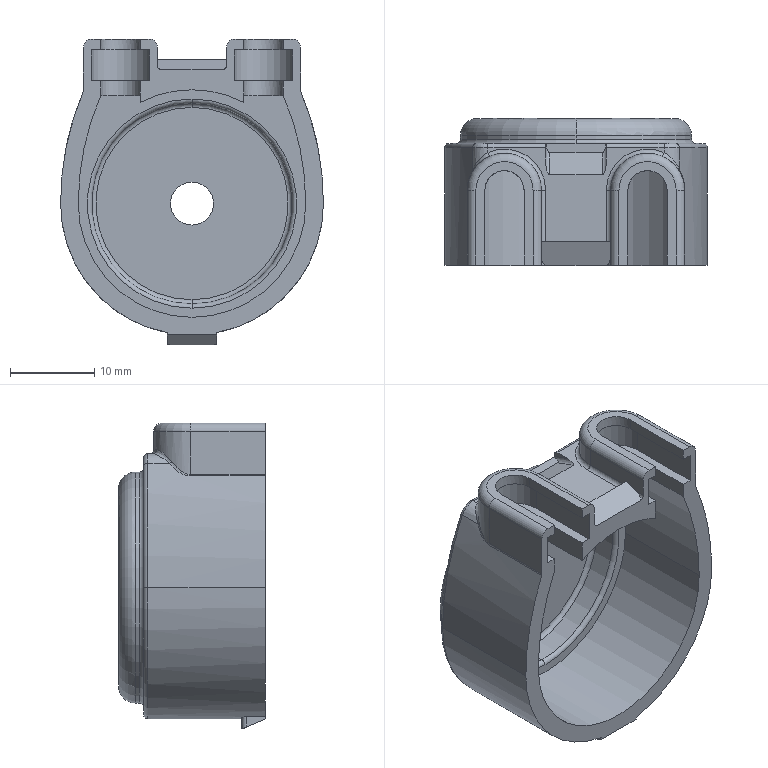Part | SolidWorks | features BaseBody 1 | 1 solid | 103 faces | box 31.23 x 17.45 x 36.34 mm | volume 4500 mm3 | plane 41 | cylinder 39 | torus 19 | spline 4 | commonest cylinder face diameters 1 x12 2 x4 4.67 x4 4 x2 5.1 x2 7 x2